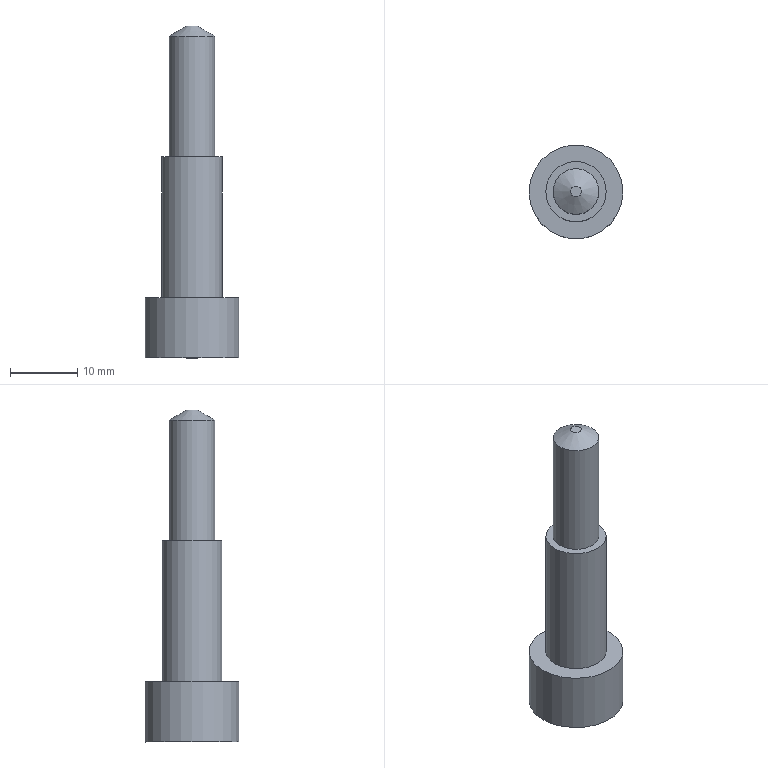Part | STEP file | solid 19 | 1 solid | 8 faces | box 14 x 14 x 49.5 mm | volume 3399 mm3 | plane 4 | cylinder 3 | cone 1 | commonest cylinder face diameters 6.8 x1 9 x1 14 x1